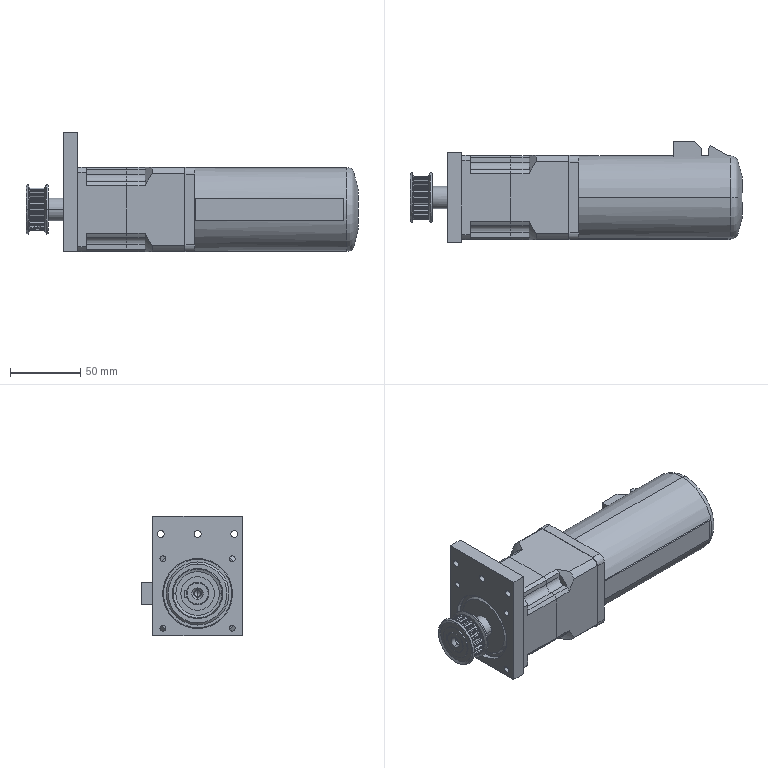Part | NX | 5 solids | 499 faces | box 237 x 72 x 85 mm | volume 619297 mm3 | cylinder 323 | plane 110 | cone 56 | torus 10 | commonest cylinder face diameters 6.55 x44 0.5 x43 1.1 x42 30.87 x42 27.33 x21 69 x16